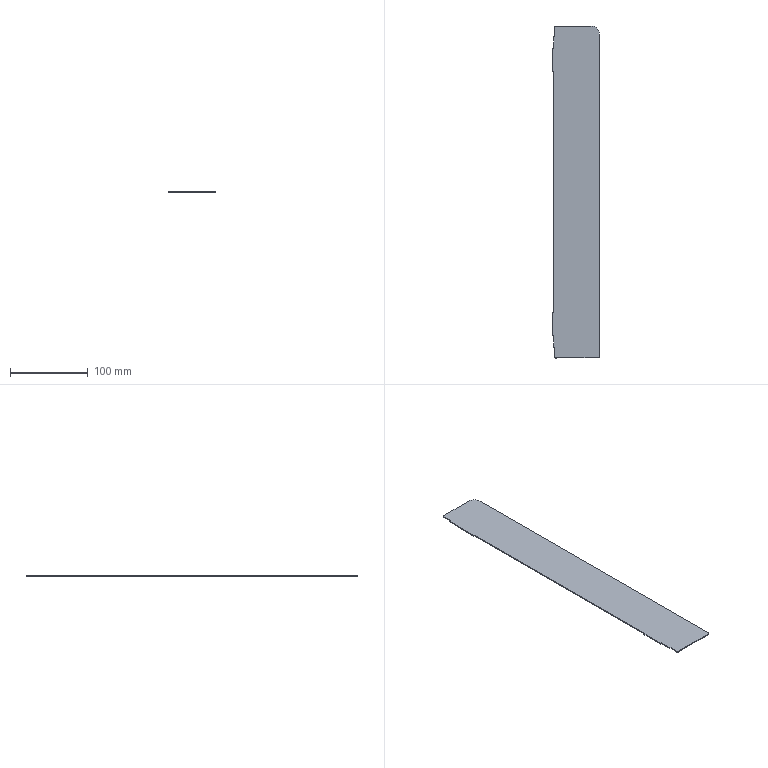Part | SolidWorks | features EdgeFlange 1, FlatPattern 1, SMBaseFlange 1, SheetMetal 1 | 1 solid | 22 faces | box 60 x 427.6 x 1.2 mm | volume 30186 mm3 | plane 18 | cylinder 4 | commonest cylinder face diameters 3 x3 21.6 x1
STEP:
#1=CARTESIAN_POINT('',(-60.,-185.,0.));
#2=VERTEX_POINT('',#1);
#3=CARTESIAN_POINT('',(-60.,-200.,0.));
#4=VERTEX_POINT('',#3);
#5=CARTESIAN_POINT('',(-60.,-185.,0.));
#6=DIRECTION('',(0.,-1.,0.));
#7=VECTOR('',#6,1000.);
#8=LINE('',#5,#7);
#9=EDGE_CURVE('',#2,#4,#8,.T.);
#10=ORIENTED_EDGE('',*,*,#9,.F.);
#11=CARTESIAN_POINT('',(-60.,-185.,-1.2));
#12=VERTEX_POINT('',#11);
#13=CARTESIAN_POINT('',(-60.,-185.,-1.2));
#14=DIRECTION('',(0.,0.,1.));
#15=VECTOR('',#14,1000.);
#16=LINE('',#13,#15);
#17=EDGE_CURVE('',#12,#2,#16,.T.);
#18=ORIENTED_EDGE('',*,*,#17,.F.);
#19=CARTESIAN_POINT('',(-60.,-200.,-1.2));
#20=VERTEX_POINT('',#19);
#21=CARTESIAN_POINT('',(-60.,-185.,-1.2));
#22=DIRECTION('',(0.,-1.,0.));
#23=VECTOR('',#22,1000.);
#24=LINE('',#21,#23);
#25=EDGE_CURVE('',#12,#20,#24,.T.);
#26=ORIENTED_EDGE('',*,*,#25,.T.);
#27=CARTESIAN_POINT('',(-60.,-200.,-1.2));
#28=DIRECTION('',(0.,0.,1.));
#29=VECTOR('',#28,1000.);
#30=LINE('',#27,#29);
#31=EDGE_CURVE('',#20,#4,#30,.T.);
#32=ORIENTED_EDGE('',*,*,#31,.T.);
#33=EDGE_LOOP('',(#10,#18,#26,#32));
#34=FACE_OUTER_BOUND('',#33,.T.);
#35=CARTESIAN_POINT('',(-60.,-185.,-1.2));
#36=DIRECTION('',(-1.,0.,0.));
#37=DIRECTION('',(0.,-1.,0.));
#38=AXIS2_PLACEMENT_3D('',#35,#36,#37);
#39=PLANE('',#38);
#40=ADVANCED_FACE('',(#34),#39,.T.);
#41=CARTESIAN_POINT('',(-61.2,-185.,0.));
#42=VERTEX_POINT('',#41);
#43=CARTESIAN_POINT('',(-60.,-185.,0.));
#44=DIRECTION('',(1.,0.,0.));
#45=VECTOR('',#44,1000.);
#46=LINE('',#43,#45);
#47=EDGE_CURVE('',#42,#2,#46,.T.);
#48=ORIENTED_EDGE('',*,*,#47,.F.);
#49=CARTESIAN_POINT('',(-61.2,-185.,-1.2));
#50=VERTEX_POINT('',#49);
#51=CARTESIAN_POINT('',(-61.2,-185.,-1.2));
#52=DIRECTION('',(0.,0.,1.));
#53=VECTOR('',#52,1000.);
#54=LINE('',#51,#53);
#55=EDGE_CURVE('',#50,#42,#54,.T.);
#56=ORIENTED_EDGE('',*,*,#55,.F.);
#57=CARTESIAN_POINT('',(-60.,-185.,-1.2));
#58=DIRECTION('',(1.,0.,0.));
#59=VECTOR('',#58,1000.);
#60=LINE('',#57,#59);
#61=EDGE_CURVE('',#50,#12,#60,.T.);
#62=ORIENTED_EDGE('',*,*,#61,.T.);
#63=ORIENTED_EDGE('',*,*,#17,.T.);
#64=EDGE_LOOP('',(#48,#56,#62,#63));
#65=FACE_OUTER_BOUND('',#64,.T.);
#66=CARTESIAN_POINT('',(-60.,-185.,-1.2));
#67=DIRECTION('',(0.,-1.,0.));
#68=DIRECTION('',(0.,0.,-1.));
#69=AXIS2_PLACEMENT_3D('',#66,#67,#68);
#70=PLANE('',#69);
#71=ADVANCED_FACE('',(#65),#70,.T.);
#72=CARTESIAN_POINT('',(-61.2,-155.,0.));
#73=VERTEX_POINT('',#72);
#74=CARTESIAN_POINT('',(-61.2,-185.,0.));
#75=DIRECTION('',(0.,-1.,0.));
#76=VECTOR('',#75,1000.);
#77=LINE('',#74,#76);
#78=EDGE_CURVE('',#73,#42,#77,.T.);
#79=ORIENTED_EDGE('',*,*,#78,.F.);
#80=CARTESIAN_POINT('',(-61.2,-155.,-1.2));
#81=VERTEX_POINT('',#80);
#82=CARTESIAN_POINT('',(-61.2,-155.,-1.2));
#83=DIRECTION('',(0.,0.,1.));
#84=VECTOR('',#83,1000.);
#85=LINE('',#82,#84);
#86=EDGE_CURVE('',#81,#73,#85,.T.);
#87=ORIENTED_EDGE('',*,*,#86,.F.);
#88=CARTESIAN_POINT('',(-61.2,-185.,-1.2));
#89=DIRECTION('',(0.,-1.,0.));
#90=VECTOR('',#89,1000.);
#91=LINE('',#88,#90);
#92=EDGE_CURVE('',#81,#50,#91,.T.);
#93=ORIENTED_EDGE('',*,*,#92,.T.);
#94=ORIENTED_EDGE('',*,*,#55,.T.);
#95=EDGE_LOOP('',(#79,#87,#93,#94));
#96=FACE_OUTER_BOUND('',#95,.T.);
#97=CARTESIAN_POINT('',(-61.2,-185.,-1.2));
#98=DIRECTION('',(-1.,0.,0.));
#99=DIRECTION('',(0.,0.,1.));
#100=AXIS2_PLACEMENT_3D('',#97,#98,#99);
#101=PLANE('',#100);
#102=ADVANCED_FACE('',(#96),#101,.T.);
#103=CARTESIAN_POINT('',(-60.,-155.,0.));
#104=VERTEX_POINT('',#103);
#105=CARTESIAN_POINT('',(-61.2,-155.,0.));
#106=DIRECTION('',(-1.,0.,0.));
#107=VECTOR('',#106,1000.);
#108=LINE('',#105,#107);
#109=EDGE_CURVE('',#104,#73,#108,.T.);
#110=ORIENTED_EDGE('',*,*,#109,.F.);
#111=CARTESIAN_POINT('',(-60.,-155.,-1.2));
#112=VERTEX_POINT('',#111);
#113=CARTESIAN_POINT('',(-60.,-155.,-1.2));
#114=DIRECTION('',(0.,0.,1.));
#115=VECTOR('',#114,1000.);
#116=LINE('',#113,#115);
#117=EDGE_CURVE('',#112,#104,#116,.T.);
#118=ORIENTED_EDGE('',*,*,#117,.F.);
#119=CARTESIAN_POINT('',(-61.2,-155.,-1.2));
#120=DIRECTION('',(-1.,0.,0.));
#121=VECTOR('',#120,1000.);
#122=LINE('',#119,#121);
#123=EDGE_CURVE('',#112,#81,#122,.T.);
#124=ORIENTED_EDGE('',*,*,#123,.T.);
#125=ORIENTED_EDGE('',*,*,#86,.T.);
#126=EDGE_LOOP('',(#110,#118,#124,#125));
#127=FACE_OUTER_BOUND('',#126,.T.);
#128=CARTESIAN_POINT('',(-61.2,-155.,-1.2));
#129=DIRECTION('',(0.,1.,0.));
#130=DIRECTION('',(0.,0.,1.));
#131=AXIS2_PLACEMENT_3D('',#128,#129,#130);
#132=PLANE('',#131);
#133=ADVANCED_FACE('',(#127),#132,.T.);
#134=CARTESIAN_POINT('',(-60.,155.,0.));
#135=VERTEX_POINT('',#134);
#136=CARTESIAN_POINT('',(-60.,155.,0.));
#137=DIRECTION('',(0.,-1.,0.));
#138=VECTOR('',#137,1000.);
#139=LINE('',#136,#138);
#140=EDGE_CURVE('',#135,#104,#139,.T.);
#141=ORIENTED_EDGE('',*,*,#140,.F.);
#142=CARTESIAN_POINT('',(-60.,155.,-1.2));
#143=VERTEX_POINT('',#142);
#144=CARTESIAN_POINT('',(-60.,155.,-1.2));
#145=DIRECTION('',(0.,0.,1.));
#146=VECTOR('',#145,1000.);
#147=LINE('',#144,#146);
#148=EDGE_CURVE('',#143,#135,#147,.T.);
#149=ORIENTED_EDGE('',*,*,#148,.F.);
#150=CARTESIAN_POINT('',(-60.,155.,-1.2));
#151=DIRECTION('',(0.,-1.,0.));
#152=VECTOR('',#151,1000.);
#153=LINE('',#150,#152);
#154=EDGE_CURVE('',#143,#112,#153,.T.);
#155=ORIENTED_EDGE('',*,*,#154,.T.);
#156=ORIENTED_EDGE('',*,*,#117,.T.);
#157=EDGE_LOOP('',(#141,#149,#155,#156));
#158=FACE_OUTER_BOUND('',#157,.T.);
#159=CARTESIAN_POINT('',(-60.,155.,-1.2));
#160=DIRECTION('',(-1.,0.,0.));
#161=DIRECTION('',(0.,-1.,0.));
#162=AXIS2_PLACEMENT_3D('',#159,#160,#161);
#163=PLANE('',#162);
#164=ADVANCED_FACE('',(#158),#163,.T.);
#165=CARTESIAN_POINT('',(-61.2,155.,0.));
#166=VERTEX_POINT('',#165);
#167=CARTESIAN_POINT('',(-61.2,155.,0.));
#168=DIRECTION('',(1.,0.,0.));
#169=VECTOR('',#168,1000.);
#170=LINE('',#167,#169);
#171=EDGE_CURVE('',#166,#135,#170,.T.);
#172=ORIENTED_EDGE('',*,*,#171,.F.);
#173=CARTESIAN_POINT('',(-61.2,155.,-1.2));
#174=VERTEX_POINT('',#173);
#175=CARTESIAN_POINT('',(-61.2,155.,-1.2));
#176=DIRECTION('',(0.,0.,1.));
#177=VECTOR('',#176,1000.);
#178=LINE('',#175,#177);
#179=EDGE_CURVE('',#174,#166,#178,.T.);
#180=ORIENTED_EDGE('',*,*,#179,.F.);
#181=CARTESIAN_POINT('',(-61.2,155.,-1.2));
#182=DIRECTION('',(1.,0.,0.));
#183=VECTOR('',#182,1000.);
#184=LINE('',#181,#183);
#185=EDGE_CURVE('',#174,#143,#184,.T.);
#186=ORIENTED_EDGE('',*,*,#185,.T.);
#187=ORIENTED_EDGE('',*,*,#148,.T.);
#188=EDGE_LOOP('',(#172,#180,#186,#187));
#189=FACE_OUTER_BOUND('',#188,.T.);
#190=CARTESIAN_POINT('',(-61.2,155.,-1.2));
#191=DIRECTION('',(0.,-1.,0.));
#192=DIRECTION('',(0.,0.,-1.));
#193=AXIS2_PLACEMENT_3D('',#190,#191,#192);
#194=PLANE('',#193);
#195=ADVANCED_FACE('',(#189),#194,.T.);
#196=CARTESIAN_POINT('',(-61.2,185.,0.));
#197=VERTEX_POINT('',#196);
#198=CARTESIAN_POINT('',(-61.2,185.,0.));
#199=DIRECTION('',(0.,-1.,0.));
#200=VECTOR('',#199,1000.);
#201=LINE('',#198,#200);
#202=EDGE_CURVE('',#197,#166,#201,.T.);
#203=ORIENTED_EDGE('',*,*,#202,.F.);
#204=CARTESIAN_POINT('',(-61.2,185.,-1.2));
#205=VERTEX_POINT('',#204);
#206=CARTESIAN_POINT('',(-61.2,185.,-1.2));
#207=DIRECTION('',(0.,0.,1.));
#208=VECTOR('',#207,1000.);
#209=LINE('',#206,#208);
#210=EDGE_CURVE('',#205,#197,#209,.T.);
#211=ORIENTED_EDGE('',*,*,#210,.F.);
#212=CARTESIAN_POINT('',(-61.2,185.,-1.2));
#213=DIRECTION('',(0.,-1.,0.));
#214=VECTOR('',#213,1000.);
#215=LINE('',#212,#214);
#216=EDGE_CURVE('',#205,#174,#215,.T.);
#217=ORIENTED_EDGE('',*,*,#216,.T.);
#218=ORIENTED_EDGE('',*,*,#179,.T.);
#219=EDGE_LOOP('',(#203,#211,#217,#218));
#220=FACE_OUTER_BOUND('',#219,.T.);
#221=CARTESIAN_POINT('',(-61.2,185.,-1.2));
#222=DIRECTION('',(-1.,0.,0.));
#223=DIRECTION('',(0.,-1.,0.));
#224=AXIS2_PLACEMENT_3D('',#221,#222,#223);
#225=PLANE('',#224);
#226=ADVANCED_FACE('',(#220),#225,.T.);
#227=CARTESIAN_POINT('',(-60.,185.,0.));
#228=VERTEX_POINT('',#227);
#229=CARTESIAN_POINT('',(-60.,185.,0.));
#230=DIRECTION('',(-1.,0.,0.));
#231=VECTOR('',#230,1000.);
#232=LINE('',#229,#231);
#233=EDGE_CURVE('',#228,#197,#232,.T.);
#234=ORIENTED_EDGE('',*,*,#233,.F.);
#235=CARTESIAN_POINT('',(-60.,185.,-1.2));
#236=VERTEX_POINT('',#235);
#237=CARTESIAN_POINT('',(-60.,185.,-1.2));
#238=DIRECTION('',(0.,0.,1.));
#239=VECTOR('',#238,1000.);
#240=LINE('',#237,#239);
#241=EDGE_CURVE('',#236,#228,#240,.T.);
#242=ORIENTED_EDGE('',*,*,#241,.F.);
#243=CARTESIAN_POINT('',(-60.,185.,-1.2));
#244=DIRECTION('',(-1.,0.,0.));
#245=VECTOR('',#244,1000.);
#246=LINE('',#243,#245);
#247=EDGE_CURVE('',#236,#205,#246,.T.);
#248=ORIENTED_EDGE('',*,*,#247,.T.);
#249=ORIENTED_EDGE('',*,*,#210,.T.);
#250=EDGE_LOOP('',(#234,#242,#248,#249));
#251=FACE_OUTER_BOUND('',#250,.T.);
#252=CARTESIAN_POINT('',(-60.,185.,-1.2));
#253=DIRECTION('',(0.,1.,0.));
#254=DIRECTION('',(0.,0.,1.));
#255=AXIS2_PLACEMENT_3D('',#252,#253,#254);
#256=PLANE('',#255);
#257=ADVANCED_FACE('',(#251),#256,.T.);
#258=CARTESIAN_POINT('',(-60.,200.,0.));
#259=VERTEX_POINT('',#258);
#260=CARTESIAN_POINT('',(-60.,200.,0.));
#261=DIRECTION('',(0.,-1.,0.));
#262=VECTOR('',#261,1000.);
#263=LINE('',#260,#262);
#264=EDGE_CURVE('',#259,#228,#263,.T.);
#265=ORIENTED_EDGE('',*,*,#264,.F.);
#266=CARTESIAN_POINT('',(-60.,200.,-1.2));
#267=VERTEX_POINT('',#266);
#268=CARTESIAN_POINT('',(-60.,200.,-1.2));
#269=DIRECTION('',(0.,0.,1.));
#270=VECTOR('',#269,1000.);
#271=LINE('',#268,#270);
#272=EDGE_CURVE('',#267,#259,#271,.T.);
#273=ORIENTED_EDGE('',*,*,#272,.F.);
#274=CARTESIAN_POINT('',(-60.,200.,-1.2));
#275=DIRECTION('',(0.,-1.,0.));
#276=VECTOR('',#275,1000.);
#277=LINE('',#274,#276);
#278=EDGE_CURVE('',#267,#236,#277,.T.);
#279=ORIENTED_EDGE('',*,*,#278,.T.);
#280=ORIENTED_EDGE('',*,*,#241,.T.);
#281=EDGE_LOOP('',(#265,#273,#279,#280));
#282=FACE_OUTER_BOUND('',#281,.T.);
#283=CARTESIAN_POINT('',(-60.,200.,-1.2));
#284=DIRECTION('',(-1.,0.,0.));
#285=DIRECTION('',(0.,0.,1.));
#286=AXIS2_PLACEMENT_3D('',#283,#284,#285);
#287=PLANE('',#286);
#288=ADVANCED_FACE('',(#282),#287,.T.);
#289=CARTESIAN_POINT('',(-58.8,200.,0.));
#290=VERTEX_POINT('',#289);
#291=CARTESIAN_POINT('',(-58.8,200.,0.));
#292=DIRECTION('',(-1.,0.,0.));
#293=VECTOR('',#292,1000.);
#294=LINE('',#291,#293);
#295=EDGE_CURVE('',#290,#259,#294,.T.);
#296=ORIENTED_EDGE('',*,*,#295,.F.);
#297=CARTESIAN_POINT('',(-58.8,200.,-1.2));
#298=VERTEX_POINT('',#297);
#299=CARTESIAN_POINT('',(-58.8,200.,-1.2));
#300=DIRECTION('',(0.,0.,1.));
#301=VECTOR('',#300,1000.);
#302=LINE('',#299,#301);
#303=EDGE_CURVE('',#298,#290,#302,.T.);
#304=ORIENTED_EDGE('',*,*,#303,.F.);
#305=CARTESIAN_POINT('',(-58.8,200.,-1.2));
#306=DIRECTION('',(-1.,0.,0.));
#307=VECTOR('',#306,1000.);
#308=LINE('',#305,#307);
#309=EDGE_CURVE('',#298,#267,#308,.T.);
#310=ORIENTED_EDGE('',*,*,#309,.T.);
#311=ORIENTED_EDGE('',*,*,#272,.T.);
#312=EDGE_LOOP('',(#296,#304,#310,#311));
#313=FACE_OUTER_BOUND('',#312,.T.);
#314=CARTESIAN_POINT('',(-58.8,200.,-1.2));
#315=DIRECTION('',(0.,1.,0.));
#316=DIRECTION('',(0.,0.,1.));
#317=AXIS2_PLACEMENT_3D('',#314,#315,#316);
#318=PLANE('',#317);
#319=ADVANCED_FACE('',(#313),#318,.T.);
#320=CARTESIAN_POINT('',(-58.8,212.3,0.));
#321=VERTEX_POINT('',#320);
#322=CARTESIAN_POINT('',(-58.8,200.,0.));
#323=DIRECTION('',(0.,-1.,0.));
#324=VECTOR('',#323,1000.);
#325=LINE('',#322,#324);
#326=EDGE_CURVE('',#321,#290,#325,.T.);
#327=ORIENTED_EDGE('',*,*,#326,.F.);
#328=CARTESIAN_POINT('',(-58.8,212.3,-1.2));
#329=VERTEX_POINT('',#328);
#330=CARTESIAN_POINT('',(-58.8,212.3,-1.2));
#331=DIRECTION('',(0.,0.,1.));
#332=VECTOR('',#331,1000.);
#333=LINE('',#330,#332);
#334=EDGE_CURVE('',#329,#321,#333,.T.);
#335=ORIENTED_EDGE('',*,*,#334,.F.);
#336=CARTESIAN_POINT('',(-58.8,200.,-1.2));
#337=DIRECTION('',(0.,-1.,0.));
#338=VECTOR('',#337,1000.);
#339=LINE('',#336,#338);
#340=EDGE_CURVE('',#329,#298,#339,.T.);
#341=ORIENTED_EDGE('',*,*,#340,.T.);
#342=ORIENTED_EDGE('',*,*,#303,.T.);
#343=EDGE_LOOP('',(#327,#335,#341,#342));
#344=FACE_OUTER_BOUND('',#343,.T.);
#345=CARTESIAN_POINT('',(-58.8,200.,-1.2));
#346=DIRECTION('',(-1.,0.,0.));
#347=DIRECTION('',(0.,-1.,0.));
#348=AXIS2_PLACEMENT_3D('',#345,#346,#347);
#349=PLANE('',#348);
#350=ADVANCED_FACE('',(#344),#349,.T.);
#351=CARTESIAN_POINT('',(-57.3,213.8,0.));
#352=VERTEX_POINT('',#351);
#353=CARTESIAN_POINT('',(-57.3,212.3,0.));
#354=DIRECTION('',(0.,0.,1.));
#355=DIRECTION('',(1.,0.,0.));
#356=AXIS2_PLACEMENT_3D('',#353,#354,#355);
#357=CIRCLE('',#356,1.5);
#358=EDGE_CURVE('',#352,#321,#357,.T.);
#359=ORIENTED_EDGE('',*,*,#358,.F.);
#360=CARTESIAN_POINT('',(-57.3,213.8,-1.2));
#361=VERTEX_POINT('',#360);
#362=CARTESIAN_POINT('',(-57.3,213.8,-1.2));
#363=DIRECTION('',(0.,0.,1.));
#364=VECTOR('',#363,1000.);
#365=LINE('',#362,#364);
#366=EDGE_CURVE('',#361,#352,#365,.T.);
#367=ORIENTED_EDGE('',*,*,#366,.F.);
#368=CARTESIAN_POINT('',(-57.3,212.3,-1.2));
#369=DIRECTION('',(0.,0.,1.));
#370=DIRECTION('',(1.,0.,0.));
#371=AXIS2_PLACEMENT_3D('',#368,#369,#370);
#372=CIRCLE('',#371,1.5);
#373=EDGE_CURVE('',#361,#329,#372,.T.);
#374=ORIENTED_EDGE('',*,*,#373,.T.);
#375=ORIENTED_EDGE('',*,*,#334,.T.);
#376=EDGE_LOOP('',(#359,#367,#374,#375));
#377=FACE_OUTER_BOUND('',#376,.T.);
#378=CARTESIAN_POINT('',(-57.3,212.3,-1.2));
#379=DIRECTION('',(0.,0.,1.));
#380=DIRECTION('',(1.,0.,0.));
#381=AXIS2_PLACEMENT_3D('',#378,#379,#380);
#382=CYLINDRICAL_SURFACE('',#381,1.5);
#383=ADVANCED_FACE('',(#377),#382,.T.);
#384=CARTESIAN_POINT('',(-12.,213.8,0.));
#385=VERTEX_POINT('',#384);
#386=CARTESIAN_POINT('',(-57.3,213.8,0.));
#387=DIRECTION('',(-1.,0.,0.));
#388=VECTOR('',#387,1000.);
#389=LINE('',#386,#388);
#390=EDGE_CURVE('',#385,#352,#389,.T.);
#391=ORIENTED_EDGE('',*,*,#390,.F.);
#392=CARTESIAN_POINT('',(-12.,213.8,-1.2));
#393=VERTEX_POINT('',#392);
#394=CARTESIAN_POINT('',(-12.,213.8,-1.2));
#395=DIRECTION('',(0.,0.,1.));
#396=VECTOR('',#395,1000.);
#397=LINE('',#394,#396);
#398=EDGE_CURVE('',#393,#385,#397,.T.);
#399=ORIENTED_EDGE('',*,*,#398,.F.);
#400=CARTESIAN_POINT('',(-57.3,213.8,-1.2));
#401=DIRECTION('',(-1.,0.,0.));
#402=VECTOR('',#401,1000.);
#403=LINE('',#400,#402);
#404=EDGE_CURVE('',#393,#361,#403,.T.);
#405=ORIENTED_EDGE('',*,*,#404,.T.);
#406=ORIENTED_EDGE('',*,*,#366,.T.);
#407=EDGE_LOOP('',(#391,#399,#405,#406));
#408=FACE_OUTER_BOUND('',#407,.T.);
#409=CARTESIAN_POINT('',(-57.3,213.8,-1.2));
#410=DIRECTION('',(0.,1.,0.));
#411=DIRECTION('',(-1.,0.,0.));
#412=AXIS2_PLACEMENT_3D('',#409,#410,#411);
#413=PLANE('',#412);
#414=ADVANCED_FACE('',(#408),#413,.T.);
#415=CARTESIAN_POINT('',(-1.2,203.,0.));
#416=VERTEX_POINT('',#415);
#417=CARTESIAN_POINT('',(-12.,203.,0.));
#418=DIRECTION('',(0.,0.,1.));
#419=DIRECTION('',(1.,0.,0.));
#420=AXIS2_PLACEMENT_3D('',#417,#418,#419);
#421=CIRCLE('',#420,10.8);
#422=EDGE_CURVE('',#416,#385,#421,.T.);
#423=ORIENTED_EDGE('',*,*,#422,.F.);
#424=CARTESIAN_POINT('',(-1.2,203.,-1.2));
#425=VERTEX_POINT('',#424);
#426=CARTESIAN_POINT('',(-1.2,203.,-1.2));
#427=DIRECTION('',(0.,0.,1.));
#428=VECTOR('',#427,1000.);
#429=LINE('',#426,#428);
#430=EDGE_CURVE('',#425,#416,#429,.T.);
#431=ORIENTED_EDGE('',*,*,#430,.F.);
#432=CARTESIAN_POINT('',(-12.,203.,-1.2));
#433=DIRECTION('',(0.,0.,1.));
#434=DIRECTION('',(1.,0.,0.));
#435=AXIS2_PLACEMENT_3D('',#432,#433,#434);
#436=CIRCLE('',#435,10.8);
#437=EDGE_CURVE('',#425,#393,#436,.T.);
#438=ORIENTED_EDGE('',*,*,#437,.T.);
#439=ORIENTED_EDGE('',*,*,#398,.T.);
#440=EDGE_LOOP('',(#423,#431,#438,#439));
#441=FACE_OUTER_BOUND('',#440,.T.);
#442=CARTESIAN_POINT('',(-12.,203.,-1.2));
#443=DIRECTION('',(0.,0.,1.));
#444=DIRECTION('',(1.,0.,0.));
#445=AXIS2_PLACEMENT_3D('',#442,#443,#444);
#446=CYLINDRICAL_SURFACE('',#445,10.8);
#447=ADVANCED_FACE('',(#441),#446,.T.);
#448=CARTESIAN_POINT('',(-1.2,-212.3,0.));
#449=VERTEX_POINT('',#448);
#450=CARTESIAN_POINT('',(-1.2,203.,0.));
#451=DIRECTION('',(0.,1.,0.));
#452=VECTOR('',#451,1000.);
#453=LINE('',#450,#452);
#454=EDGE_CURVE('',#449,#416,#453,.T.);
#455=ORIENTED_EDGE('',*,*,#454,.F.);
#456=CARTESIAN_POINT('',(-1.2,-212.3,-1.2));
#457=VERTEX_POINT('',#456);
#458=CARTESIAN_POINT('',(-1.2,-212.3,-1.2));
#459=DIRECTION('',(0.,0.,1.));
#460=VECTOR('',#459,1000.);
#461=LINE('',#458,#460);
#462=EDGE_CURVE('',#457,#449,#461,.T.);
#463=ORIENTED_EDGE('',*,*,#462,.F.);
#464=CARTESIAN_POINT('',(-1.2,203.,-1.2));
#465=DIRECTION('',(0.,1.,0.));
#466=VECTOR('',#465,1000.);
#467=LINE('',#464,#466);
#468=EDGE_CURVE('',#457,#425,#467,.T.);
#469=ORIENTED_EDGE('',*,*,#468,.T.);
#470=ORIENTED_EDGE('',*,*,#430,.T.);
#471=EDGE_LOOP('',(#455,#463,#469,#470));
#472=FACE_OUTER_BOUND('',#471,.T.);
#473=CARTESIAN_POINT('',(-1.2,203.,-1.2));
#474=DIRECTION('',(1.,0.,0.));
#475=DIRECTION('',(0.,1.,0.));
#476=AXIS2_PLACEMENT_3D('',#473,#474,#475);
#477=PLANE('',#476);
#478=ADVANCED_FACE('',(#472),#477,.T.);
#479=CARTESIAN_POINT('',(-2.7,-213.8,0.));
#480=VERTEX_POINT('',#479);
#481=CARTESIAN_POINT('',(-2.7,-212.3,0.));
#482=DIRECTION('',(0.,0.,1.));
#483=DIRECTION('',(1.,0.,0.));
#484=AXIS2_PLACEMENT_3D('',#481,#482,#483);
#485=CIRCLE('',#484,1.5);
#486=EDGE_CURVE('',#480,#449,#485,.T.);
#487=ORIENTED_EDGE('',*,*,#486,.F.);
#488=CARTESIAN_POINT('',(-2.7,-213.8,-1.2));
#489=VERTEX_POINT('',#488);
#490=CARTESIAN_POINT('',(-2.7,-213.8,-1.2));
#491=DIRECTION('',(0.,0.,1.));
#492=VECTOR('',#491,1000.);
#493=LINE('',#490,#492);
#494=EDGE_CURVE('',#489,#480,#493,.T.);
#495=ORIENTED_EDGE('',*,*,#494,.F.);
#496=CARTESIAN_POINT('',(-2.7,-212.3,-1.2));
#497=DIRECTION('',(0.,0.,1.));
#498=DIRECTION('',(1.,0.,0.));
#499=AXIS2_PLACEMENT_3D('',#496,#497,#498);
#500=CIRCLE('',#499,1.5);
#501=EDGE_CURVE('',#489,#457,#500,.T.);
#502=ORIENTED_EDGE('',*,*,#501,.T.);
#503=ORIENTED_EDGE('',*,*,#462,.T.);
#504=EDGE_LOOP('',(#487,#495,#502,#503));
#505=FACE_OUTER_BOUND('',#504,.T.);
#506=CARTESIAN_POINT('',(-2.7,-212.3,-1.2));
#507=DIRECTION('',(0.,0.,1.));
#508=DIRECTION('',(1.,0.,0.));
#509=AXIS2_PLACEMENT_3D('',#506,#507,#508);
#510=CYLINDRICAL_SURFACE('',#509,1.5);
#511=ADVANCED_FACE('',(#505),#510,.T.);
#512=CARTESIAN_POINT('',(-57.3,-213.8,0.));
#513=VERTEX_POINT('',#512);
#514=CARTESIAN_POINT('',(-2.7,-213.8,0.));
#515=DIRECTION('',(1.,0.,0.));
#516=VECTOR('',#515,1000.);
#517=LINE('',#514,#516);
#518=EDGE_CURVE('',#513,#480,#517,.T.);
#519=ORIENTED_EDGE('',*,*,#518,.F.);
#520=CARTESIAN_POINT('',(-57.3,-213.8,-1.2));
#521=VERTEX_POINT('',#520);
#522=CARTESIAN_POINT('',(-57.3,-213.8,-1.2));
#523=DIRECTION('',(0.,0.,1.));
#524=VECTOR('',#523,1000.);
#525=LINE('',#522,#524);
#526=EDGE_CURVE('',#521,#513,#525,.T.);
#527=ORIENTED_EDGE('',*,*,#526,.F.);
#528=CARTESIAN_POINT('',(-2.7,-213.8,-1.2));
#529=DIRECTION('',(1.,0.,0.));
#530=VECTOR('',#529,1000.);
#531=LINE('',#528,#530);
#532=EDGE_CURVE('',#521,#489,#531,.T.);
#533=ORIENTED_EDGE('',*,*,#532,.T.);
#534=ORIENTED_EDGE('',*,*,#494,.T.);
#535=EDGE_LOOP('',(#519,#527,#533,#534));
#536=FACE_OUTER_BOUND('',#535,.T.);
#537=CARTESIAN_POINT('',(-2.7,-213.8,-1.2));
#538=DIRECTION('',(0.,-1.,0.));
#539=DIRECTION('',(1.,0.,0.));
#540=AXIS2_PLACEMENT_3D('',#537,#538,#539);
#541=PLANE('',#540);
#542=ADVANCED_FACE('',(#536),#541,.T.);
#543=CARTESIAN_POINT('',(-58.8,-212.3,0.));
#544=VERTEX_POINT('',#543);
#545=CARTESIAN_POINT('',(-57.3,-212.3,0.));
#546=DIRECTION('',(0.,0.,1.));
#547=DIRECTION('',(1.,0.,0.));
#548=AXIS2_PLACEMENT_3D('',#545,#546,#547);
#549=CIRCLE('',#548,1.5);
#550=EDGE_CURVE('',#544,#513,#549,.T.);
#551=ORIENTED_EDGE('',*,*,#550,.F.);
#552=CARTESIAN_POINT('',(-58.8,-212.3,-1.2));
#553=VERTEX_POINT('',#552);
#554=CARTESIAN_POINT('',(-58.8,-212.3,-1.2));
#555=DIRECTION('',(0.,0.,1.));
#556=VECTOR('',#555,1000.);
#557=LINE('',#554,#556);
#558=EDGE_CURVE('',#553,#544,#557,.T.);
#559=ORIENTED_EDGE('',*,*,#558,.F.);
#560=CARTESIAN_POINT('',(-57.3,-212.3,-1.2));
#561=DIRECTION('',(0.,0.,1.));
#562=DIRECTION('',(1.,0.,0.));
#563=AXIS2_PLACEMENT_3D('',#560,#561,#562);
#564=CIRCLE('',#563,1.5);
#565=EDGE_CURVE('',#553,#521,#564,.T.);
#566=ORIENTED_EDGE('',*,*,#565,.T.);
#567=ORIENTED_EDGE('',*,*,#526,.T.);
#568=EDGE_LOOP('',(#551,#559,#566,#567));
#569=FACE_OUTER_BOUND('',#568,.T.);
#570=CARTESIAN_POINT('',(-57.3,-212.3,-1.2));
#571=DIRECTION('',(0.,0.,1.));
#572=DIRECTION('',(1.,0.,0.));
#573=AXIS2_PLACEMENT_3D('',#570,#571,#572);
#574=CYLINDRICAL_SURFACE('',#573,1.5);
#575=ADVANCED_FACE('',(#569),#574,.T.);
#576=CARTESIAN_POINT('',(-58.8,-200.,0.));
#577=VERTEX_POINT('',#576);
#578=CARTESIAN_POINT('',(-58.8,-212.3,0.));
#579=DIRECTION('',(0.,-1.,0.));
#580=VECTOR('',#579,1000.);
#581=LINE('',#578,#580);
#582=EDGE_CURVE('',#577,#544,#581,.T.);
#583=ORIENTED_EDGE('',*,*,#582,.F.);
#584=CARTESIAN_POINT('',(-58.8,-200.,-1.2));
#585=VERTEX_POINT('',#584);
#586=CARTESIAN_POINT('',(-58.8,-200.,-1.2));
#587=DIRECTION('',(0.,0.,1.));
#588=VECTOR('',#587,1000.);
#589=LINE('',#586,#588);
#590=EDGE_CURVE('',#585,#577,#589,.T.);
#591=ORIENTED_EDGE('',*,*,#590,.F.);
#592=CARTESIAN_POINT('',(-58.8,-212.3,-1.2));
#593=DIRECTION('',(0.,-1.,0.));
#594=VECTOR('',#593,1000.);
#595=LINE('',#592,#594);
#596=EDGE_CURVE('',#585,#553,#595,.T.);
#597=ORIENTED_EDGE('',*,*,#596,.T.);
#598=ORIENTED_EDGE('',*,*,#558,.T.);
#599=EDGE_LOOP('',(#583,#591,#597,#598));
#600=FACE_OUTER_BOUND('',#599,.T.);
#601=CARTESIAN_POINT('',(-58.8,-212.3,-1.2));
#602=DIRECTION('',(-1.,0.,0.));
#603=DIRECTION('',(0.,-1.,0.));
#604=AXIS2_PLACEMENT_3D('',#601,#602,#603);
#605=PLANE('',#604);
#606=ADVANCED_FACE('',(#600),#605,.T.);
#607=CARTESIAN_POINT('',(-60.,-200.,0.));
#608=DIRECTION('',(1.,0.,0.));
#609=VECTOR('',#608,1000.);
#610=LINE('',#607,#609);
#611=EDGE_CURVE('',#4,#577,#610,.T.);
#612=ORIENTED_EDGE('',*,*,#611,.F.);
#613=ORIENTED_EDGE('',*,*,#31,.F.);
#614=CARTESIAN_POINT('',(-60.,-200.,-1.2));
#615=DIRECTION('',(1.,0.,0.));
#616=VECTOR('',#615,1000.);
#617=LINE('',#614,#616);
#618=EDGE_CURVE('',#20,#585,#617,.T.);
#619=ORIENTED_EDGE('',*,*,#618,.T.);
#620=ORIENTED_EDGE('',*,*,#590,.T.);
#621=EDGE_LOOP('',(#612,#613,#619,#620));
#622=FACE_OUTER_BOUND('',#621,.T.);
#623=CARTESIAN_POINT('',(-60.,-200.,-1.2));
#624=DIRECTION('',(0.,-1.,0.));
#625=DIRECTION('',(0.,0.,-1.));
#626=AXIS2_PLACEMENT_3D('',#623,#624,#625);
#627=PLANE('',#626);
#628=ADVANCED_FACE('',(#622),#627,.T.);
#629=ORIENTED_EDGE('',*,*,#25,.F.);
#630=ORIENTED_EDGE('',*,*,#61,.F.);
#631=ORIENTED_EDGE('',*,*,#92,.F.);
#632=ORIENTED_EDGE('',*,*,#123,.F.);
#633=ORIENTED_EDGE('',*,*,#154,.F.);
#634=ORIENTED_EDGE('',*,*,#185,.F.);
#635=ORIENTED_EDGE('',*,*,#216,.F.);
#636=ORIENTED_EDGE('',*,*,#247,.F.);
#637=ORIENTED_EDGE('',*,*,#278,.F.);
#638=ORIENTED_EDGE('',*,*,#309,.F.);
#639=ORIENTED_EDGE('',*,*,#340,.F.);
#640=ORIENTED_EDGE('',*,*,#373,.F.);
#641=ORIENTED_EDGE('',*,*,#404,.F.);
#642=ORIENTED_EDGE('',*,*,#437,.F.);
#643=ORIENTED_EDGE('',*,*,#468,.F.);
#644=ORIENTED_EDGE('',*,*,#501,.F.);
#645=ORIENTED_EDGE('',*,*,#532,.F.);
#646=ORIENTED_EDGE('',*,*,#565,.F.);
#647=ORIENTED_EDGE('',*,*,#596,.F.);
#648=ORIENTED_EDGE('',*,*,#618,.F.);
#649=EDGE_LOOP('',(#629,#630,#631,#632,#633,#634,#635,#636,#637,#638,#639,#640,#641,#642,#643,#644,#645,#646,#647,#648));
#650=FACE_OUTER_BOUND('',#649,.T.);
#651=CARTESIAN_POINT('',(-57.3,-212.3,-1.2));
#652=DIRECTION('',(0.,0.,1.));
#653=DIRECTION('',(1.,0.,0.));
#654=AXIS2_PLACEMENT_3D('',#651,#652,#653);
#655=PLANE('',#654);
#656=ADVANCED_FACE('',(#650),#655,.F.);
#657=ORIENTED_EDGE('',*,*,#9,.T.);
#658=ORIENTED_EDGE('',*,*,#611,.T.);
#659=ORIENTED_EDGE('',*,*,#582,.T.);
#660=ORIENTED_EDGE('',*,*,#550,.T.);
#661=ORIENTED_EDGE('',*,*,#518,.T.);
#662=ORIENTED_EDGE('',*,*,#486,.T.);
#663=ORIENTED_EDGE('',*,*,#454,.T.);
#664=ORIENTED_EDGE('',*,*,#422,.T.);
#665=ORIENTED_EDGE('',*,*,#390,.T.);
#666=ORIENTED_EDGE('',*,*,#358,.T.);
#667=ORIENTED_EDGE('',*,*,#326,.T.);
#668=ORIENTED_EDGE('',*,*,#295,.T.);
#669=ORIENTED_EDGE('',*,*,#264,.T.);
#670=ORIENTED_EDGE('',*,*,#233,.T.);
#671=ORIENTED_EDGE('',*,*,#202,.T.);
#672=ORIENTED_EDGE('',*,*,#171,.T.);
#673=ORIENTED_EDGE('',*,*,#140,.T.);
#674=ORIENTED_EDGE('',*,*,#109,.T.);
#675=ORIENTED_EDGE('',*,*,#78,.T.);
#676=ORIENTED_EDGE('',*,*,#47,.T.);
#677=EDGE_LOOP('',(#657,#658,#659,#660,#661,#662,#663,#664,#665,#666,#667,#668,#669,#670,#671,#672,#673,#674,#675,#676));
#678=FACE_OUTER_BOUND('',#677,.T.);
#679=CARTESIAN_POINT('',(-57.3,-212.3,0.));
#680=DIRECTION('',(0.,0.,1.));
#681=DIRECTION('',(1.,0.,0.));
#682=AXIS2_PLACEMENT_3D('',#679,#680,#681);
#683=PLANE('',#682);
#684=ADVANCED_FACE('',(#678),#683,.T.);
#685=CLOSED_SHELL('',(#40,#71,#102,#133,#164,#195,#226,#257,#288,#319,#350,#383,#414,#447,#478,#511,#542,#575,#606,#628,#656,#684));
#686=MANIFOLD_SOLID_BREP('',#685);
#687=CARTESIAN_POINT('',(0.,0.,0.));
#688=DIRECTION('',(0.,0.,1.));
#689=DIRECTION('',(1.,0.,0.));
#690=AXIS2_PLACEMENT_3D('',#687,#688,#689);
#691=(LENGTH_UNIT()NAMED_UNIT(*)SI_UNIT(.MILLI.,.METRE.));
#692=UNCERTAINTY_MEASURE_WITH_UNIT(LENGTH_MEASURE(0.00001),#691,'','');
#693=(NAMED_UNIT(*)PLANE_ANGLE_UNIT()SI_UNIT($,.RADIAN.));
#694=(NAMED_UNIT(*)SI_UNIT($,.STERADIAN.)SOLID_ANGLE_UNIT());
#695=(GEOMETRIC_REPRESENTATION_CONTEXT(3)GLOBAL_UNCERTAINTY_ASSIGNED_CONTEXT((#692))GLOBAL_UNIT_ASSIGNED_CONTEXT((#691,#693,#694))REPRESENTATION_CONTEXT('',''));
#696=ADVANCED_BREP_SHAPE_REPRESENTATION('',(#686,#690),#695);